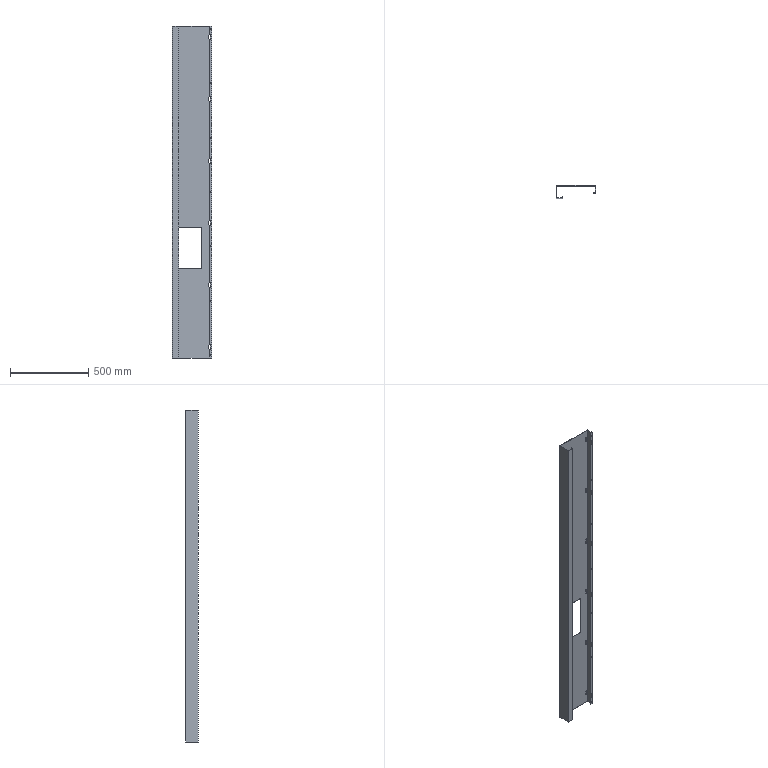Part | SolidWorks | features ICE 6, Cut 4, EdgeFlange 2, MirrorPattern 2, Fillet 1, FlatPattern 1, SMBaseFlange 1, SheetMetal 1 | 1 solid | 132 faces | box 250 x 80 x 2116 mm | volume 1045484 mm3 | plane 76 | cylinder 56 | commonest cylinder face diameters 6.2 x28 9 x18 1 x5 3.4 x5